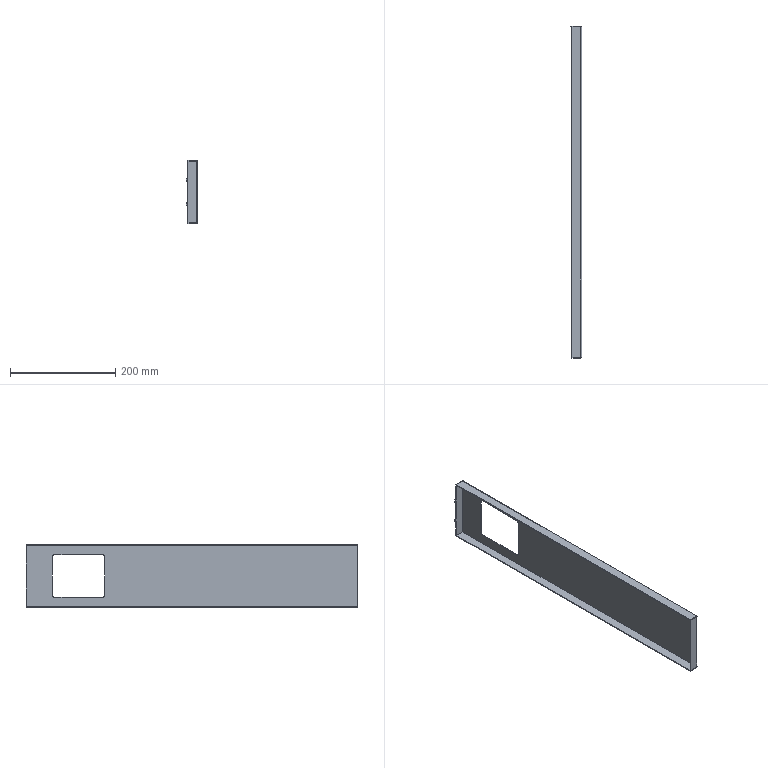Part | STEP file | HESS-408-70-15W-W-21-cabinet lower right outer plate | 1 solid | 54 faces | box 21.5 x 631 x 120 mm | volume 138943 mm3 | plane 42 | cylinder 12 | commonest cylinder face diameters 0.2 x4 3.2 x4 6 x4